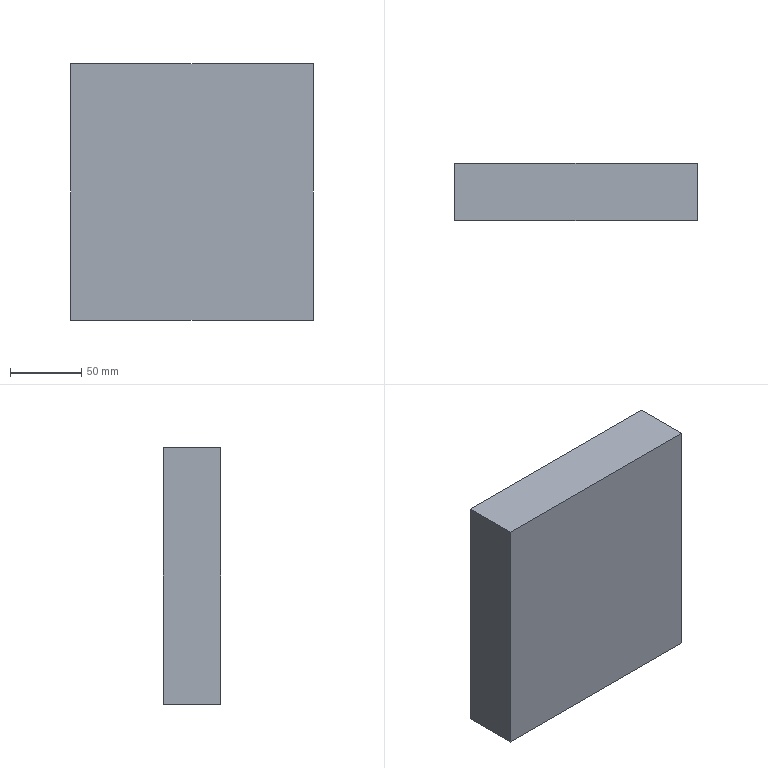Part | SolidWorks | features Extrusion 1 | 1 solid | 6 faces | box 170 x 40 x 180 mm | volume 1224000 mm3 | plane 6
STEP:
#1=CARTESIAN_POINT('',(85.,0.,90.));
#2=VERTEX_POINT('',#1);
#3=CARTESIAN_POINT('',(85.,0.,-90.));
#4=VERTEX_POINT('',#3);
#5=CARTESIAN_POINT('',(85.,0.,90.));
#6=DIRECTION('',(0.,0.,-1.));
#7=VECTOR('',#6,1000.);
#8=LINE('',#5,#7);
#9=EDGE_CURVE('',#2,#4,#8,.T.);
#10=ORIENTED_EDGE('',*,*,#9,.T.);
#11=CARTESIAN_POINT('',(85.,40.,-90.));
#12=VERTEX_POINT('',#11);
#13=CARTESIAN_POINT('',(85.,40.,-90.));
#14=DIRECTION('',(0.,-1.,0.));
#15=VECTOR('',#14,1000.);
#16=LINE('',#13,#15);
#17=EDGE_CURVE('',#12,#4,#16,.T.);
#18=ORIENTED_EDGE('',*,*,#17,.F.);
#19=CARTESIAN_POINT('',(85.,40.,90.));
#20=VERTEX_POINT('',#19);
#21=CARTESIAN_POINT('',(85.,40.,90.));
#22=DIRECTION('',(0.,0.,-1.));
#23=VECTOR('',#22,1000.);
#24=LINE('',#21,#23);
#25=EDGE_CURVE('',#20,#12,#24,.T.);
#26=ORIENTED_EDGE('',*,*,#25,.F.);
#27=CARTESIAN_POINT('',(85.,40.,90.));
#28=DIRECTION('',(0.,-1.,0.));
#29=VECTOR('',#28,1000.);
#30=LINE('',#27,#29);
#31=EDGE_CURVE('',#20,#2,#30,.T.);
#32=ORIENTED_EDGE('',*,*,#31,.T.);
#33=EDGE_LOOP('',(#10,#18,#26,#32));
#34=FACE_OUTER_BOUND('',#33,.T.);
#35=CARTESIAN_POINT('',(85.,40.,90.));
#36=DIRECTION('',(-1.,0.,0.));
#37=DIRECTION('',(0.,0.,1.));
#38=AXIS2_PLACEMENT_3D('',#35,#36,#37);
#39=PLANE('',#38);
#40=ADVANCED_FACE('',(#34),#39,.F.);
#41=CARTESIAN_POINT('',(-85.,0.,-90.));
#42=VERTEX_POINT('',#41);
#43=CARTESIAN_POINT('',(-85.,0.,-90.));
#44=DIRECTION('',(-1.,0.,0.));
#45=VECTOR('',#44,1000.);
#46=LINE('',#43,#45);
#47=EDGE_CURVE('',#4,#42,#46,.T.);
#48=ORIENTED_EDGE('',*,*,#47,.T.);
#49=CARTESIAN_POINT('',(-85.,40.,-90.));
#50=VERTEX_POINT('',#49);
#51=CARTESIAN_POINT('',(-85.,40.,-90.));
#52=DIRECTION('',(0.,-1.,0.));
#53=VECTOR('',#52,1000.);
#54=LINE('',#51,#53);
#55=EDGE_CURVE('',#50,#42,#54,.T.);
#56=ORIENTED_EDGE('',*,*,#55,.F.);
#57=CARTESIAN_POINT('',(-85.,40.,-90.));
#58=DIRECTION('',(-1.,0.,0.));
#59=VECTOR('',#58,1000.);
#60=LINE('',#57,#59);
#61=EDGE_CURVE('',#12,#50,#60,.T.);
#62=ORIENTED_EDGE('',*,*,#61,.F.);
#63=ORIENTED_EDGE('',*,*,#17,.T.);
#64=EDGE_LOOP('',(#48,#56,#62,#63));
#65=FACE_OUTER_BOUND('',#64,.T.);
#66=CARTESIAN_POINT('',(-85.,40.,-90.));
#67=DIRECTION('',(0.,0.,1.));
#68=DIRECTION('',(1.,0.,0.));
#69=AXIS2_PLACEMENT_3D('',#66,#67,#68);
#70=PLANE('',#69);
#71=ADVANCED_FACE('',(#65),#70,.F.);
#72=CARTESIAN_POINT('',(-85.,0.,90.));
#73=VERTEX_POINT('',#72);
#74=CARTESIAN_POINT('',(-85.,0.,90.));
#75=DIRECTION('',(0.,0.,1.));
#76=VECTOR('',#75,1000.);
#77=LINE('',#74,#76);
#78=EDGE_CURVE('',#42,#73,#77,.T.);
#79=ORIENTED_EDGE('',*,*,#78,.T.);
#80=CARTESIAN_POINT('',(-85.,40.,90.));
#81=VERTEX_POINT('',#80);
#82=CARTESIAN_POINT('',(-85.,40.,90.));
#83=DIRECTION('',(0.,-1.,0.));
#84=VECTOR('',#83,1000.);
#85=LINE('',#82,#84);
#86=EDGE_CURVE('',#81,#73,#85,.T.);
#87=ORIENTED_EDGE('',*,*,#86,.F.);
#88=CARTESIAN_POINT('',(-85.,40.,90.));
#89=DIRECTION('',(0.,0.,1.));
#90=VECTOR('',#89,1000.);
#91=LINE('',#88,#90);
#92=EDGE_CURVE('',#50,#81,#91,.T.);
#93=ORIENTED_EDGE('',*,*,#92,.F.);
#94=ORIENTED_EDGE('',*,*,#55,.T.);
#95=EDGE_LOOP('',(#79,#87,#93,#94));
#96=FACE_OUTER_BOUND('',#95,.T.);
#97=CARTESIAN_POINT('',(-85.,40.,90.));
#98=DIRECTION('',(1.,0.,0.));
#99=DIRECTION('',(0.,0.,-1.));
#100=AXIS2_PLACEMENT_3D('',#97,#98,#99);
#101=PLANE('',#100);
#102=ADVANCED_FACE('',(#96),#101,.F.);
#103=CARTESIAN_POINT('',(-85.,0.,90.));
#104=DIRECTION('',(1.,0.,0.));
#105=VECTOR('',#104,1000.);
#106=LINE('',#103,#105);
#107=EDGE_CURVE('',#73,#2,#106,.T.);
#108=ORIENTED_EDGE('',*,*,#107,.T.);
#109=ORIENTED_EDGE('',*,*,#31,.F.);
#110=CARTESIAN_POINT('',(-85.,40.,90.));
#111=DIRECTION('',(1.,0.,0.));
#112=VECTOR('',#111,1000.);
#113=LINE('',#110,#112);
#114=EDGE_CURVE('',#81,#20,#113,.T.);
#115=ORIENTED_EDGE('',*,*,#114,.F.);
#116=ORIENTED_EDGE('',*,*,#86,.T.);
#117=EDGE_LOOP('',(#108,#109,#115,#116));
#118=FACE_OUTER_BOUND('',#117,.T.);
#119=CARTESIAN_POINT('',(-85.,40.,90.));
#120=DIRECTION('',(0.,0.,-1.));
#121=DIRECTION('',(-1.,0.,0.));
#122=AXIS2_PLACEMENT_3D('',#119,#120,#121);
#123=PLANE('',#122);
#124=ADVANCED_FACE('',(#118),#123,.F.);
#125=ORIENTED_EDGE('',*,*,#25,.T.);
#126=ORIENTED_EDGE('',*,*,#61,.T.);
#127=ORIENTED_EDGE('',*,*,#92,.T.);
#128=ORIENTED_EDGE('',*,*,#114,.T.);
#129=EDGE_LOOP('',(#125,#126,#127,#128));
#130=FACE_OUTER_BOUND('',#129,.T.);
#131=CARTESIAN_POINT('',(0.,40.,0.));
#132=DIRECTION('',(0.,-1.,0.));
#133=DIRECTION('',(0.,0.,-1.));
#134=AXIS2_PLACEMENT_3D('',#131,#132,#133);
#135=PLANE('',#134);
#136=ADVANCED_FACE('',(#130),#135,.F.);
#137=ORIENTED_EDGE('',*,*,#9,.F.);
#138=ORIENTED_EDGE('',*,*,#107,.F.);
#139=ORIENTED_EDGE('',*,*,#78,.F.);
#140=ORIENTED_EDGE('',*,*,#47,.F.);
#141=EDGE_LOOP('',(#137,#138,#139,#140));
#142=FACE_OUTER_BOUND('',#141,.T.);
#143=CARTESIAN_POINT('',(0.,0.,0.));
#144=DIRECTION('',(0.,-1.,0.));
#145=DIRECTION('',(0.,0.,-1.));
#146=AXIS2_PLACEMENT_3D('',#143,#144,#145);
#147=PLANE('',#146);
#148=ADVANCED_FACE('',(#142),#147,.T.);
#149=CLOSED_SHELL('',(#40,#71,#102,#124,#136,#148));
#150=MANIFOLD_SOLID_BREP('',#149);
#151=CARTESIAN_POINT('',(0.,0.,0.));
#152=DIRECTION('',(0.,0.,1.));
#153=DIRECTION('',(1.,0.,0.));
#154=AXIS2_PLACEMENT_3D('',#151,#152,#153);
#155=(LENGTH_UNIT()NAMED_UNIT(*)SI_UNIT(.MILLI.,.METRE.));
#156=UNCERTAINTY_MEASURE_WITH_UNIT(LENGTH_MEASURE(0.00001),#155,'','');
#157=(NAMED_UNIT(*)PLANE_ANGLE_UNIT()SI_UNIT($,.RADIAN.));
#158=(NAMED_UNIT(*)SI_UNIT($,.STERADIAN.)SOLID_ANGLE_UNIT());
#159=(GEOMETRIC_REPRESENTATION_CONTEXT(3)GLOBAL_UNCERTAINTY_ASSIGNED_CONTEXT((#156))GLOBAL_UNIT_ASSIGNED_CONTEXT((#155,#157,#158))REPRESENTATION_CONTEXT('',''));
#160=ADVANCED_BREP_SHAPE_REPRESENTATION('',(#150,#154),#159);